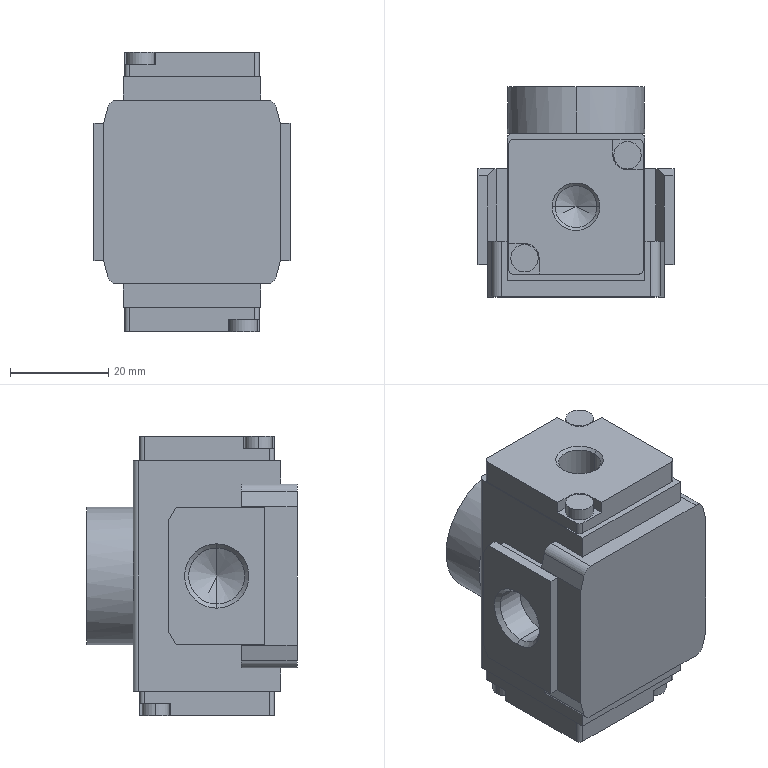Part | STEP file | AR20-02G(0)_BODY_HI | 1 solid | 131 faces | box 40 x 42.9 x 57 mm | volume 61556 mm3 | plane 81 | cylinder 38 | cone 12 | commonest cylinder face diameters 2 x10 5.6 x8 4 x4 6 x4 11.445 x4 24 x3